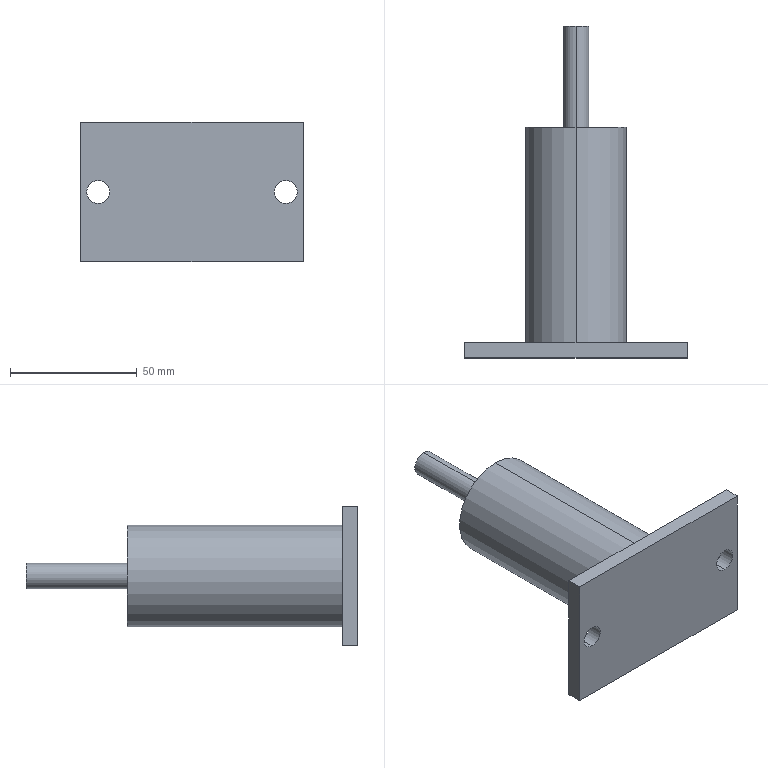Part | SolidWorks | features ICE 2, Extrusion 1, HoleWzd 1 | 1 solid | 16 faces | box 88 x 131 x 55 mm | volume 138232 mm3 | cylinder 8 | plane 8 | commonest cylinder face diameters 9 x4 10 x2 40 x2
STEP:
#1=CARTESIAN_POINT('',(0.,131.,5.));
#2=VERTEX_POINT('',#1);
#3=CARTESIAN_POINT('',(0.,131.,-5.));
#4=VERTEX_POINT('',#3);
#5=CARTESIAN_POINT('',(0.,131.,0.));
#6=DIRECTION('',(0.,1.,0.));
#7=DIRECTION('',(0.,0.,1.));
#8=AXIS2_PLACEMENT_3D('',#5,#6,#7);
#9=CIRCLE('',#8,5.);
#10=EDGE_CURVE('',#2,#4,#9,.T.);
#11=ORIENTED_EDGE('',*,*,#10,.F.);
#12=CARTESIAN_POINT('',(0.,91.,5.));
#13=VERTEX_POINT('',#12);
#14=CARTESIAN_POINT('',(0.,131.,5.));
#15=DIRECTION('',(0.,-1.,0.));
#16=VECTOR('',#15,1000.);
#17=LINE('',#14,#16);
#18=EDGE_CURVE('',#2,#13,#17,.T.);
#19=ORIENTED_EDGE('',*,*,#18,.T.);
#20=CARTESIAN_POINT('',(0.,91.,-5.));
#21=VERTEX_POINT('',#20);
#22=CARTESIAN_POINT('',(0.,91.,0.));
#23=DIRECTION('',(0.,1.,0.));
#24=DIRECTION('',(0.,0.,1.));
#25=AXIS2_PLACEMENT_3D('',#22,#23,#24);
#26=CIRCLE('',#25,5.);
#27=EDGE_CURVE('',#13,#21,#26,.T.);
#28=ORIENTED_EDGE('',*,*,#27,.T.);
#29=CARTESIAN_POINT('',(0.,131.,-5.));
#30=DIRECTION('',(0.,-1.,0.));
#31=VECTOR('',#30,1000.);
#32=LINE('',#29,#31);
#33=EDGE_CURVE('',#4,#21,#32,.T.);
#34=ORIENTED_EDGE('',*,*,#33,.F.);
#35=EDGE_LOOP('',(#11,#19,#28,#34));
#36=FACE_OUTER_BOUND('',#35,.T.);
#37=CARTESIAN_POINT('',(0.,131.,0.));
#38=DIRECTION('',(0.,-1.,0.));
#39=DIRECTION('',(0.,0.,-1.));
#40=AXIS2_PLACEMENT_3D('',#37,#38,#39);
#41=CYLINDRICAL_SURFACE('',#40,5.);
#42=ADVANCED_FACE('',(#36),#41,.T.);
#43=CARTESIAN_POINT('',(0.,91.,20.));
#44=VERTEX_POINT('',#43);
#45=CARTESIAN_POINT('',(0.,91.,-20.));
#46=VERTEX_POINT('',#45);
#47=CARTESIAN_POINT('',(0.,91.,0.));
#48=DIRECTION('',(0.,1.,0.));
#49=DIRECTION('',(0.,0.,1.));
#50=AXIS2_PLACEMENT_3D('',#47,#48,#49);
#51=CIRCLE('',#50,20.);
#52=EDGE_CURVE('',#44,#46,#51,.T.);
#53=ORIENTED_EDGE('',*,*,#52,.F.);
#54=CARTESIAN_POINT('',(0.,6.,20.));
#55=VERTEX_POINT('',#54);
#56=CARTESIAN_POINT('',(0.,91.,20.));
#57=DIRECTION('',(0.,-1.,0.));
#58=VECTOR('',#57,1000.);
#59=LINE('',#56,#58);
#60=EDGE_CURVE('',#44,#55,#59,.T.);
#61=ORIENTED_EDGE('',*,*,#60,.T.);
#62=CARTESIAN_POINT('',(0.,6.,-20.));
#63=VERTEX_POINT('',#62);
#64=CARTESIAN_POINT('',(0.,6.,0.));
#65=DIRECTION('',(0.,1.,0.));
#66=DIRECTION('',(0.,0.,-1.));
#67=AXIS2_PLACEMENT_3D('',#64,#65,#66);
#68=CIRCLE('',#67,20.);
#69=EDGE_CURVE('',#55,#63,#68,.T.);
#70=ORIENTED_EDGE('',*,*,#69,.T.);
#71=CARTESIAN_POINT('',(0.,91.,-20.));
#72=DIRECTION('',(0.,-1.,0.));
#73=VECTOR('',#72,1000.);
#74=LINE('',#71,#73);
#75=EDGE_CURVE('',#46,#63,#74,.T.);
#76=ORIENTED_EDGE('',*,*,#75,.F.);
#77=EDGE_LOOP('',(#53,#61,#70,#76));
#78=FACE_OUTER_BOUND('',#77,.T.);
#79=CARTESIAN_POINT('',(0.,91.,0.));
#80=DIRECTION('',(0.,-1.,0.));
#81=DIRECTION('',(0.,0.,-1.));
#82=AXIS2_PLACEMENT_3D('',#79,#80,#81);
#83=CYLINDRICAL_SURFACE('',#82,20.);
#84=ADVANCED_FACE('',(#78),#83,.T.);
#85=CARTESIAN_POINT('',(-37.,0.,-4.5));
#86=VERTEX_POINT('',#85);
#87=CARTESIAN_POINT('',(-37.,0.,4.5));
#88=VERTEX_POINT('',#87);
#89=CARTESIAN_POINT('',(-37.,0.,0.));
#90=DIRECTION('',(0.,1.,0.));
#91=DIRECTION('',(0.,0.,1.));
#92=AXIS2_PLACEMENT_3D('',#89,#90,#91);
#93=CIRCLE('',#92,4.5);
#94=EDGE_CURVE('',#86,#88,#93,.T.);
#95=ORIENTED_EDGE('',*,*,#94,.F.);
#96=CARTESIAN_POINT('',(-37.,6.,-4.5));
#97=VERTEX_POINT('',#96);
#98=CARTESIAN_POINT('',(-37.,6.,-4.5));
#99=DIRECTION('',(0.,1.,0.));
#100=VECTOR('',#99,1000.);
#101=LINE('',#98,#100);
#102=EDGE_CURVE('',#86,#97,#101,.T.);
#103=ORIENTED_EDGE('',*,*,#102,.T.);
#104=CARTESIAN_POINT('',(-37.,6.,4.5));
#105=VERTEX_POINT('',#104);
#106=CARTESIAN_POINT('',(-37.,6.,0.));
#107=DIRECTION('',(0.,1.,0.));
#108=DIRECTION('',(0.,0.,1.));
#109=AXIS2_PLACEMENT_3D('',#106,#107,#108);
#110=CIRCLE('',#109,4.5);
#111=EDGE_CURVE('',#97,#105,#110,.T.);
#112=ORIENTED_EDGE('',*,*,#111,.T.);
#113=CARTESIAN_POINT('',(-37.,6.,4.5));
#114=DIRECTION('',(0.,1.,0.));
#115=VECTOR('',#114,1000.);
#116=LINE('',#113,#115);
#117=EDGE_CURVE('',#88,#105,#116,.T.);
#118=ORIENTED_EDGE('',*,*,#117,.F.);
#119=EDGE_LOOP('',(#95,#103,#112,#118));
#120=FACE_OUTER_BOUND('',#119,.T.);
#121=CARTESIAN_POINT('',(-37.,6.,0.));
#122=DIRECTION('',(0.,1.,0.));
#123=DIRECTION('',(0.,0.,1.));
#124=AXIS2_PLACEMENT_3D('',#121,#122,#123);
#125=CYLINDRICAL_SURFACE('',#124,4.5);
#126=ADVANCED_FACE('',(#120),#125,.F.);
#127=CARTESIAN_POINT('',(37.,0.,-4.5));
#128=VERTEX_POINT('',#127);
#129=CARTESIAN_POINT('',(37.,0.,4.5));
#130=VERTEX_POINT('',#129);
#131=CARTESIAN_POINT('',(37.,0.,0.));
#132=DIRECTION('',(0.,1.,0.));
#133=DIRECTION('',(0.,0.,1.));
#134=AXIS2_PLACEMENT_3D('',#131,#132,#133);
#135=CIRCLE('',#134,4.5);
#136=EDGE_CURVE('',#128,#130,#135,.T.);
#137=ORIENTED_EDGE('',*,*,#136,.F.);
#138=CARTESIAN_POINT('',(37.,6.,-4.5));
#139=VERTEX_POINT('',#138);
#140=CARTESIAN_POINT('',(37.,6.,-4.5));
#141=DIRECTION('',(0.,1.,0.));
#142=VECTOR('',#141,1000.);
#143=LINE('',#140,#142);
#144=EDGE_CURVE('',#128,#139,#143,.T.);
#145=ORIENTED_EDGE('',*,*,#144,.T.);
#146=CARTESIAN_POINT('',(37.,6.,4.5));
#147=VERTEX_POINT('',#146);
#148=CARTESIAN_POINT('',(37.,6.,0.));
#149=DIRECTION('',(0.,1.,0.));
#150=DIRECTION('',(0.,0.,1.));
#151=AXIS2_PLACEMENT_3D('',#148,#149,#150);
#152=CIRCLE('',#151,4.5);
#153=EDGE_CURVE('',#139,#147,#152,.T.);
#154=ORIENTED_EDGE('',*,*,#153,.T.);
#155=CARTESIAN_POINT('',(37.,6.,4.5));
#156=DIRECTION('',(0.,1.,0.));
#157=VECTOR('',#156,1000.);
#158=LINE('',#155,#157);
#159=EDGE_CURVE('',#130,#147,#158,.T.);
#160=ORIENTED_EDGE('',*,*,#159,.F.);
#161=EDGE_LOOP('',(#137,#145,#154,#160));
#162=FACE_OUTER_BOUND('',#161,.T.);
#163=CARTESIAN_POINT('',(37.,6.,0.));
#164=DIRECTION('',(0.,1.,0.));
#165=DIRECTION('',(0.,0.,1.));
#166=AXIS2_PLACEMENT_3D('',#163,#164,#165);
#167=CYLINDRICAL_SURFACE('',#166,4.5);
#168=ADVANCED_FACE('',(#162),#167,.F.);
#169=CARTESIAN_POINT('',(44.,0.,27.5));
#170=VERTEX_POINT('',#169);
#171=CARTESIAN_POINT('',(44.,0.,-27.5));
#172=VERTEX_POINT('',#171);
#173=CARTESIAN_POINT('',(44.,0.,27.5));
#174=DIRECTION('',(0.,0.,-1.));
#175=VECTOR('',#174,1000.);
#176=LINE('',#173,#175);
#177=EDGE_CURVE('',#170,#172,#176,.T.);
#178=ORIENTED_EDGE('',*,*,#177,.T.);
#179=CARTESIAN_POINT('',(44.,6.,-27.5));
#180=VERTEX_POINT('',#179);
#181=CARTESIAN_POINT('',(44.,6.,-27.5));
#182=DIRECTION('',(0.,-1.,0.));
#183=VECTOR('',#182,1000.);
#184=LINE('',#181,#183);
#185=EDGE_CURVE('',#180,#172,#184,.T.);
#186=ORIENTED_EDGE('',*,*,#185,.F.);
#187=CARTESIAN_POINT('',(44.,6.,27.5));
#188=VERTEX_POINT('',#187);
#189=CARTESIAN_POINT('',(44.,6.,27.5));
#190=DIRECTION('',(0.,0.,-1.));
#191=VECTOR('',#190,1000.);
#192=LINE('',#189,#191);
#193=EDGE_CURVE('',#188,#180,#192,.T.);
#194=ORIENTED_EDGE('',*,*,#193,.F.);
#195=CARTESIAN_POINT('',(44.,6.,27.5));
#196=DIRECTION('',(0.,-1.,0.));
#197=VECTOR('',#196,1000.);
#198=LINE('',#195,#197);
#199=EDGE_CURVE('',#188,#170,#198,.T.);
#200=ORIENTED_EDGE('',*,*,#199,.T.);
#201=EDGE_LOOP('',(#178,#186,#194,#200));
#202=FACE_OUTER_BOUND('',#201,.T.);
#203=CARTESIAN_POINT('',(44.,6.,27.5));
#204=DIRECTION('',(-1.,0.,0.));
#205=DIRECTION('',(0.,0.,1.));
#206=AXIS2_PLACEMENT_3D('',#203,#204,#205);
#207=PLANE('',#206);
#208=ADVANCED_FACE('',(#202),#207,.F.);
#209=CARTESIAN_POINT('',(-44.,0.,-27.5));
#210=VERTEX_POINT('',#209);
#211=CARTESIAN_POINT('',(-44.,0.,-27.5));
#212=DIRECTION('',(-1.,0.,0.));
#213=VECTOR('',#212,1000.);
#214=LINE('',#211,#213);
#215=EDGE_CURVE('',#172,#210,#214,.T.);
#216=ORIENTED_EDGE('',*,*,#215,.T.);
#217=CARTESIAN_POINT('',(-44.,6.,-27.5));
#218=VERTEX_POINT('',#217);
#219=CARTESIAN_POINT('',(-44.,6.,-27.5));
#220=DIRECTION('',(0.,-1.,0.));
#221=VECTOR('',#220,1000.);
#222=LINE('',#219,#221);
#223=EDGE_CURVE('',#218,#210,#222,.T.);
#224=ORIENTED_EDGE('',*,*,#223,.F.);
#225=CARTESIAN_POINT('',(-44.,6.,-27.5));
#226=DIRECTION('',(-1.,0.,0.));
#227=VECTOR('',#226,1000.);
#228=LINE('',#225,#227);
#229=EDGE_CURVE('',#180,#218,#228,.T.);
#230=ORIENTED_EDGE('',*,*,#229,.F.);
#231=ORIENTED_EDGE('',*,*,#185,.T.);
#232=EDGE_LOOP('',(#216,#224,#230,#231));
#233=FACE_OUTER_BOUND('',#232,.T.);
#234=CARTESIAN_POINT('',(-44.,6.,-27.5));
#235=DIRECTION('',(0.,0.,1.));
#236=DIRECTION('',(1.,0.,0.));
#237=AXIS2_PLACEMENT_3D('',#234,#235,#236);
#238=PLANE('',#237);
#239=ADVANCED_FACE('',(#233),#238,.F.);
#240=CARTESIAN_POINT('',(-44.,0.,27.5));
#241=VERTEX_POINT('',#240);
#242=CARTESIAN_POINT('',(-44.,0.,27.5));
#243=DIRECTION('',(0.,0.,1.));
#244=VECTOR('',#243,1000.);
#245=LINE('',#242,#244);
#246=EDGE_CURVE('',#210,#241,#245,.T.);
#247=ORIENTED_EDGE('',*,*,#246,.T.);
#248=CARTESIAN_POINT('',(-44.,6.,27.5));
#249=VERTEX_POINT('',#248);
#250=CARTESIAN_POINT('',(-44.,6.,27.5));
#251=DIRECTION('',(0.,-1.,0.));
#252=VECTOR('',#251,1000.);
#253=LINE('',#250,#252);
#254=EDGE_CURVE('',#249,#241,#253,.T.);
#255=ORIENTED_EDGE('',*,*,#254,.F.);
#256=CARTESIAN_POINT('',(-44.,6.,27.5));
#257=DIRECTION('',(0.,0.,1.));
#258=VECTOR('',#257,1000.);
#259=LINE('',#256,#258);
#260=EDGE_CURVE('',#218,#249,#259,.T.);
#261=ORIENTED_EDGE('',*,*,#260,.F.);
#262=ORIENTED_EDGE('',*,*,#223,.T.);
#263=EDGE_LOOP('',(#247,#255,#261,#262));
#264=FACE_OUTER_BOUND('',#263,.T.);
#265=CARTESIAN_POINT('',(-44.,6.,27.5));
#266=DIRECTION('',(1.,0.,0.));
#267=DIRECTION('',(0.,0.,-1.));
#268=AXIS2_PLACEMENT_3D('',#265,#266,#267);
#269=PLANE('',#268);
#270=ADVANCED_FACE('',(#264),#269,.F.);
#271=CARTESIAN_POINT('',(-44.,0.,27.5));
#272=DIRECTION('',(1.,0.,0.));
#273=VECTOR('',#272,1000.);
#274=LINE('',#271,#273);
#275=EDGE_CURVE('',#241,#170,#274,.T.);
#276=ORIENTED_EDGE('',*,*,#275,.T.);
#277=ORIENTED_EDGE('',*,*,#199,.F.);
#278=CARTESIAN_POINT('',(-44.,6.,27.5));
#279=DIRECTION('',(1.,0.,0.));
#280=VECTOR('',#279,1000.);
#281=LINE('',#278,#280);
#282=EDGE_CURVE('',#249,#188,#281,.T.);
#283=ORIENTED_EDGE('',*,*,#282,.F.);
#284=ORIENTED_EDGE('',*,*,#254,.T.);
#285=EDGE_LOOP('',(#276,#277,#283,#284));
#286=FACE_OUTER_BOUND('',#285,.T.);
#287=CARTESIAN_POINT('',(-44.,6.,27.5));
#288=DIRECTION('',(0.,0.,-1.));
#289=DIRECTION('',(-1.,0.,0.));
#290=AXIS2_PLACEMENT_3D('',#287,#288,#289);
#291=PLANE('',#290);
#292=ADVANCED_FACE('',(#286),#291,.F.);
#293=CARTESIAN_POINT('',(0.,6.,0.));
#294=DIRECTION('',(0.,1.,0.));
#295=DIRECTION('',(0.,0.,-1.));
#296=AXIS2_PLACEMENT_3D('',#293,#294,#295);
#297=CIRCLE('',#296,20.);
#298=EDGE_CURVE('',#63,#55,#297,.T.);
#299=ORIENTED_EDGE('',*,*,#298,.F.);
#300=ORIENTED_EDGE('',*,*,#69,.F.);
#301=EDGE_LOOP('',(#299,#300));
#302=FACE_BOUND('',#301,.T.);
#303=CARTESIAN_POINT('',(-37.,6.,0.));
#304=DIRECTION('',(0.,1.,0.));
#305=DIRECTION('',(0.,0.,1.));
#306=AXIS2_PLACEMENT_3D('',#303,#304,#305);
#307=CIRCLE('',#306,4.5);
#308=EDGE_CURVE('',#105,#97,#307,.T.);
#309=ORIENTED_EDGE('',*,*,#308,.F.);
#310=ORIENTED_EDGE('',*,*,#111,.F.);
#311=EDGE_LOOP('',(#309,#310));
#312=FACE_BOUND('',#311,.T.);
#313=CARTESIAN_POINT('',(37.,6.,0.));
#314=DIRECTION('',(0.,1.,0.));
#315=DIRECTION('',(0.,0.,1.));
#316=AXIS2_PLACEMENT_3D('',#313,#314,#315);
#317=CIRCLE('',#316,4.5);
#318=EDGE_CURVE('',#147,#139,#317,.T.);
#319=ORIENTED_EDGE('',*,*,#318,.F.);
#320=ORIENTED_EDGE('',*,*,#153,.F.);
#321=EDGE_LOOP('',(#319,#320));
#322=FACE_BOUND('',#321,.T.);
#323=ORIENTED_EDGE('',*,*,#193,.T.);
#324=ORIENTED_EDGE('',*,*,#229,.T.);
#325=ORIENTED_EDGE('',*,*,#260,.T.);
#326=ORIENTED_EDGE('',*,*,#282,.T.);
#327=EDGE_LOOP('',(#323,#324,#325,#326));
#328=FACE_OUTER_BOUND('',#327,.T.);
#329=CARTESIAN_POINT('',(0.,6.,0.));
#330=DIRECTION('',(0.,-1.,0.));
#331=DIRECTION('',(0.,0.,-1.));
#332=AXIS2_PLACEMENT_3D('',#329,#330,#331);
#333=PLANE('',#332);
#334=ADVANCED_FACE('',(#302,#312,#322,#328),#333,.F.);
#335=CARTESIAN_POINT('',(-37.,0.,0.));
#336=DIRECTION('',(0.,1.,0.));
#337=DIRECTION('',(0.,0.,1.));
#338=AXIS2_PLACEMENT_3D('',#335,#336,#337);
#339=CIRCLE('',#338,4.5);
#340=EDGE_CURVE('',#88,#86,#339,.T.);
#341=ORIENTED_EDGE('',*,*,#340,.T.);
#342=ORIENTED_EDGE('',*,*,#94,.T.);
#343=EDGE_LOOP('',(#341,#342));
#344=FACE_BOUND('',#343,.T.);
#345=CARTESIAN_POINT('',(37.,0.,0.));
#346=DIRECTION('',(0.,1.,0.));
#347=DIRECTION('',(0.,0.,1.));
#348=AXIS2_PLACEMENT_3D('',#345,#346,#347);
#349=CIRCLE('',#348,4.5);
#350=EDGE_CURVE('',#130,#128,#349,.T.);
#351=ORIENTED_EDGE('',*,*,#350,.T.);
#352=ORIENTED_EDGE('',*,*,#136,.T.);
#353=EDGE_LOOP('',(#351,#352));
#354=FACE_BOUND('',#353,.T.);
#355=ORIENTED_EDGE('',*,*,#177,.F.);
#356=ORIENTED_EDGE('',*,*,#275,.F.);
#357=ORIENTED_EDGE('',*,*,#246,.F.);
#358=ORIENTED_EDGE('',*,*,#215,.F.);
#359=EDGE_LOOP('',(#355,#356,#357,#358));
#360=FACE_OUTER_BOUND('',#359,.T.);
#361=CARTESIAN_POINT('',(0.,0.,0.));
#362=DIRECTION('',(0.,-1.,0.));
#363=DIRECTION('',(0.,0.,-1.));
#364=AXIS2_PLACEMENT_3D('',#361,#362,#363);
#365=PLANE('',#364);
#366=ADVANCED_FACE('',(#344,#354,#360),#365,.T.);
#367=ORIENTED_EDGE('',*,*,#144,.F.);
#368=ORIENTED_EDGE('',*,*,#350,.F.);
#369=ORIENTED_EDGE('',*,*,#159,.T.);
#370=ORIENTED_EDGE('',*,*,#318,.T.);
#371=EDGE_LOOP('',(#367,#368,#369,#370));
#372=FACE_OUTER_BOUND('',#371,.T.);
#373=CARTESIAN_POINT('',(37.,6.,0.));
#374=DIRECTION('',(0.,1.,0.));
#375=DIRECTION('',(0.,0.,1.));
#376=AXIS2_PLACEMENT_3D('',#373,#374,#375);
#377=CYLINDRICAL_SURFACE('',#376,4.5);
#378=ADVANCED_FACE('',(#372),#377,.F.);
#379=ORIENTED_EDGE('',*,*,#102,.F.);
#380=ORIENTED_EDGE('',*,*,#340,.F.);
#381=ORIENTED_EDGE('',*,*,#117,.T.);
#382=ORIENTED_EDGE('',*,*,#308,.T.);
#383=EDGE_LOOP('',(#379,#380,#381,#382));
#384=FACE_OUTER_BOUND('',#383,.T.);
#385=CARTESIAN_POINT('',(-37.,6.,0.));
#386=DIRECTION('',(0.,1.,0.));
#387=DIRECTION('',(0.,0.,1.));
#388=AXIS2_PLACEMENT_3D('',#385,#386,#387);
#389=CYLINDRICAL_SURFACE('',#388,4.5);
#390=ADVANCED_FACE('',(#384),#389,.F.);
#391=ORIENTED_EDGE('',*,*,#60,.F.);
#392=CARTESIAN_POINT('',(0.,91.,0.));
#393=DIRECTION('',(0.,1.,0.));
#394=DIRECTION('',(0.,0.,1.));
#395=AXIS2_PLACEMENT_3D('',#392,#393,#394);
#396=CIRCLE('',#395,20.);
#397=EDGE_CURVE('',#46,#44,#396,.T.);
#398=ORIENTED_EDGE('',*,*,#397,.F.);
#399=ORIENTED_EDGE('',*,*,#75,.T.);
#400=ORIENTED_EDGE('',*,*,#298,.T.);
#401=EDGE_LOOP('',(#391,#398,#399,#400));
#402=FACE_OUTER_BOUND('',#401,.T.);
#403=CARTESIAN_POINT('',(0.,91.,0.));
#404=DIRECTION('',(0.,-1.,0.));
#405=DIRECTION('',(0.,0.,-1.));
#406=AXIS2_PLACEMENT_3D('',#403,#404,#405);
#407=CYLINDRICAL_SURFACE('',#406,20.);
#408=ADVANCED_FACE('',(#402),#407,.T.);
#409=CARTESIAN_POINT('',(0.,91.,0.));
#410=DIRECTION('',(0.,1.,0.));
#411=DIRECTION('',(0.,0.,1.));
#412=AXIS2_PLACEMENT_3D('',#409,#410,#411);
#413=CIRCLE('',#412,5.);
#414=EDGE_CURVE('',#21,#13,#413,.T.);
#415=ORIENTED_EDGE('',*,*,#414,.F.);
#416=ORIENTED_EDGE('',*,*,#27,.F.);
#417=EDGE_LOOP('',(#415,#416));
#418=FACE_BOUND('',#417,.T.);
#419=ORIENTED_EDGE('',*,*,#397,.T.);
#420=ORIENTED_EDGE('',*,*,#52,.T.);
#421=EDGE_LOOP('',(#419,#420));
#422=FACE_OUTER_BOUND('',#421,.T.);
#423=CARTESIAN_POINT('',(0.,91.,0.));
#424=DIRECTION('',(0.,1.,0.));
#425=DIRECTION('',(0.,0.,1.));
#426=AXIS2_PLACEMENT_3D('',#423,#424,#425);
#427=PLANE('',#426);
#428=ADVANCED_FACE('',(#418,#422),#427,.T.);
#429=ORIENTED_EDGE('',*,*,#18,.F.);
#430=CARTESIAN_POINT('',(0.,131.,0.));
#431=DIRECTION('',(0.,1.,0.));
#432=DIRECTION('',(0.,0.,1.));
#433=AXIS2_PLACEMENT_3D('',#430,#431,#432);
#434=CIRCLE('',#433,5.);
#435=EDGE_CURVE('',#4,#2,#434,.T.);
#436=ORIENTED_EDGE('',*,*,#435,.F.);
#437=ORIENTED_EDGE('',*,*,#33,.T.);
#438=ORIENTED_EDGE('',*,*,#414,.T.);
#439=EDGE_LOOP('',(#429,#436,#437,#438));
#440=FACE_OUTER_BOUND('',#439,.T.);
#441=CARTESIAN_POINT('',(0.,131.,0.));
#442=DIRECTION('',(0.,-1.,0.));
#443=DIRECTION('',(0.,0.,-1.));
#444=AXIS2_PLACEMENT_3D('',#441,#442,#443);
#445=CYLINDRICAL_SURFACE('',#444,5.);
#446=ADVANCED_FACE('',(#440),#445,.T.);
#447=ORIENTED_EDGE('',*,*,#435,.T.);
#448=ORIENTED_EDGE('',*,*,#10,.T.);
#449=EDGE_LOOP('',(#447,#448));
#450=FACE_OUTER_BOUND('',#449,.T.);
#451=CARTESIAN_POINT('',(0.,131.,0.));
#452=DIRECTION('',(0.,1.,0.));
#453=DIRECTION('',(0.,0.,1.));
#454=AXIS2_PLACEMENT_3D('',#451,#452,#453);
#455=PLANE('',#454);
#456=ADVANCED_FACE('',(#450),#455,.T.);
#457=CLOSED_SHELL('',(#42,#84,#126,#168,#208,#239,#270,#292,#334,#366,#378,#390,#408,#428,#446,#456));
#458=MANIFOLD_SOLID_BREP('',#457);
#459=CARTESIAN_POINT('',(0.,0.,0.));
#460=DIRECTION('',(0.,0.,1.));
#461=DIRECTION('',(1.,0.,0.));
#462=AXIS2_PLACEMENT_3D('',#459,#460,#461);
#463=(LENGTH_UNIT()NAMED_UNIT(*)SI_UNIT(.MILLI.,.METRE.));
#464=UNCERTAINTY_MEASURE_WITH_UNIT(LENGTH_MEASURE(0.00001),#463,'','');
#465=(NAMED_UNIT(*)PLANE_ANGLE_UNIT()SI_UNIT($,.RADIAN.));
#466=(NAMED_UNIT(*)SI_UNIT($,.STERADIAN.)SOLID_ANGLE_UNIT());
#467=(GEOMETRIC_REPRESENTATION_CONTEXT(3)GLOBAL_UNCERTAINTY_ASSIGNED_CONTEXT((#464))GLOBAL_UNIT_ASSIGNED_CONTEXT((#463,#465,#466))REPRESENTATION_CONTEXT('',''));
#468=ADVANCED_BREP_SHAPE_REPRESENTATION('',(#458,#462),#467);